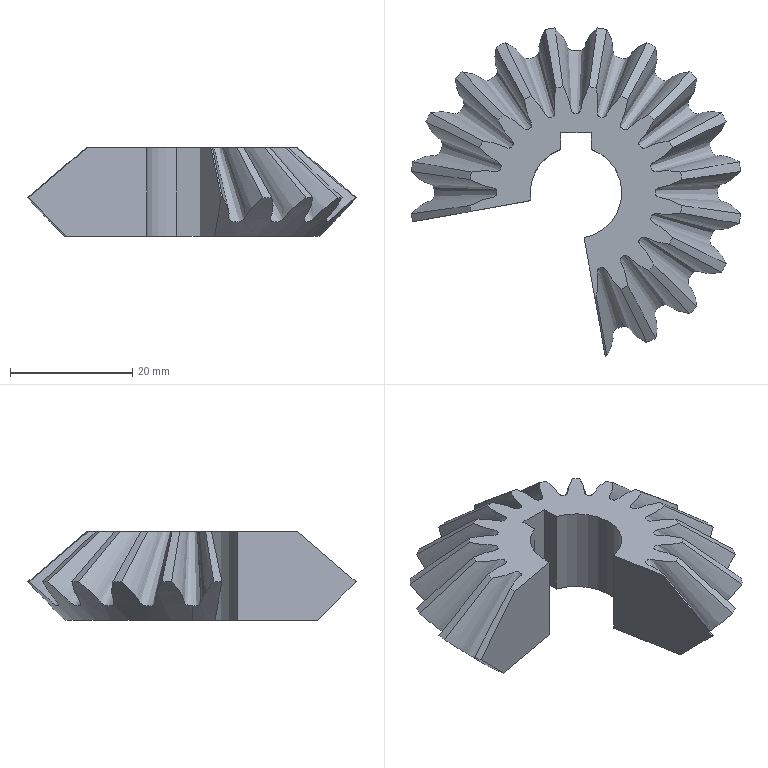Part | STEP file | Cuon T phu H01_11_Bevel01 | 1 solid | 44 faces | box 53.951 x 53.746 x 14.57 mm | volume 13339 mm3 | cone 19 | spline 15 | plane 7 | cylinder 3 | commonest cylinder face diameters 15 x3